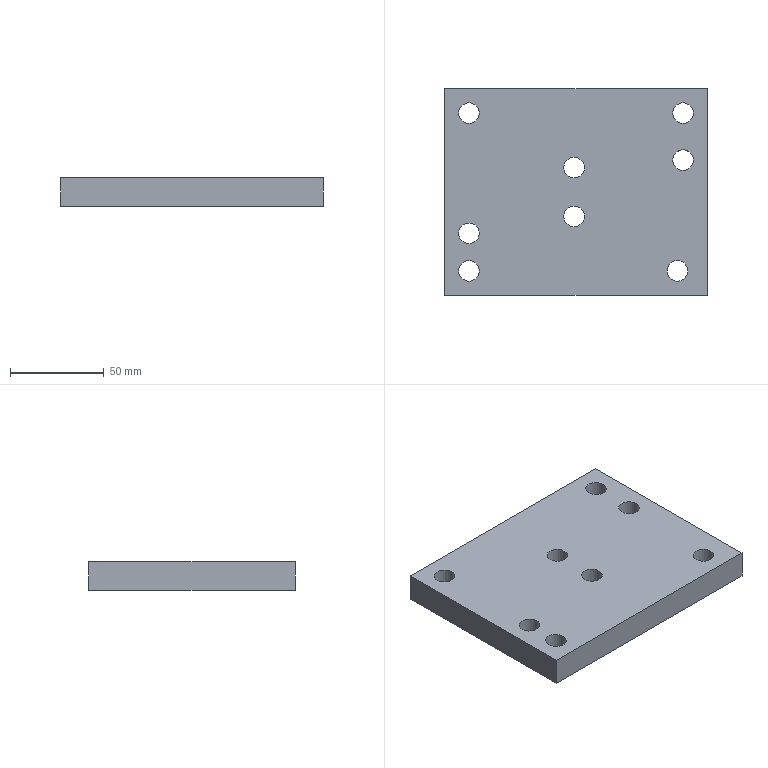Part | STEP file | 101_id682_x_t | 1 solid | 14 faces | box 140 x 110 x 15 mm | volume 219596 mm3 | cylinder 8 | plane 6 | commonest cylinder face diameters 11 x8
STEP:
#1=CARTESIAN_POINT('',(0.,0.,0.));
#2=DIRECTION('',(0.,0.,1.));
#3=DIRECTION('',(1.,0.,0.));
#4=AXIS2_PLACEMENT_3D('',#1,#2,#3);
#5=CARTESIAN_POINT('',(-791.5,35.5,105.));
#6=VERTEX_POINT('',#5);
#7=CARTESIAN_POINT('',(-791.5,35.5,90.));
#8=VERTEX_POINT('',#7);
#9=CARTESIAN_POINT('',(-791.5,35.5,95.));
#10=DIRECTION('',(0.,0.,-1.));
#11=VECTOR('',#10,1.);
#12=LINE('',#9,#11);
#13=CARTESIAN_POINT('',(-791.5,94.,95.));
#14=DIRECTION('',(-1.,0.,0.));
#15=DIRECTION('',(0.,-1.,0.));
#16=AXIS2_PLACEMENT_3D('',#13,#14,#15);
#17=PLANE('',#16);
#18=CARTESIAN_POINT('',(58.5,0.));
#19=DIRECTION('',(0.,-1.));
#20=VECTOR('',#19,1.);
#21=LINE('',#18,#20);
#22=(GEOMETRIC_REPRESENTATION_CONTEXT(2)PARAMETRIC_REPRESENTATION_CONTEXT()REPRESENTATION_CONTEXT('',''));
#23=DEFINITIONAL_REPRESENTATION('',(#21),#22);
#24=PCURVE('',#17,#23);
#25=CARTESIAN_POINT('',(-870.,35.5,95.));
#26=DIRECTION('',(0.,1.,0.));
#27=DIRECTION('',(-1.,0.,0.));
#28=AXIS2_PLACEMENT_3D('',#25,#26,#27);
#29=PLANE('',#28);
#30=CARTESIAN_POINT('',(-78.5,0.));
#31=DIRECTION('',(0.,-1.));
#32=VECTOR('',#31,1.);
#33=LINE('',#30,#32);
#34=(GEOMETRIC_REPRESENTATION_CONTEXT(2)PARAMETRIC_REPRESENTATION_CONTEXT()REPRESENTATION_CONTEXT('',''));
#35=DEFINITIONAL_REPRESENTATION('',(#33),#34);
#36=PCURVE('',#29,#35);
#37=SURFACE_CURVE('',#12,(#24,#36),.PCURVE_S1.);
#38=EDGE_CURVE('',#6,#8,#37,.T.);
#39=ORIENTED_EDGE('',*,*,#38,.T.);
#40=CARTESIAN_POINT('',(-791.5,145.5,90.));
#41=VERTEX_POINT('',#40);
#42=CARTESIAN_POINT('',(-791.5,94.,90.));
#43=DIRECTION('',(0.,-1.,0.));
#44=VECTOR('',#43,1.);
#45=LINE('',#42,#44);
#46=CARTESIAN_POINT('',(0.,-5.));
#47=DIRECTION('',(1.,0.));
#48=VECTOR('',#47,1.);
#49=LINE('',#46,#48);
#50=(GEOMETRIC_REPRESENTATION_CONTEXT(2)PARAMETRIC_REPRESENTATION_CONTEXT()REPRESENTATION_CONTEXT('',''));
#51=DEFINITIONAL_REPRESENTATION('',(#49),#50);
#52=PCURVE('',#17,#51);
#53=CARTESIAN_POINT('',(-870.,94.,90.));
#54=DIRECTION('',(0.,0.,1.));
#55=DIRECTION('',(0.,-1.,0.));
#56=AXIS2_PLACEMENT_3D('',#53,#54,#55);
#57=PLANE('',#56);
#58=CARTESIAN_POINT('',(0.,78.5));
#59=DIRECTION('',(1.,0.));
#60=VECTOR('',#59,1.);
#61=LINE('',#58,#60);
#62=(GEOMETRIC_REPRESENTATION_CONTEXT(2)PARAMETRIC_REPRESENTATION_CONTEXT()REPRESENTATION_CONTEXT('',''));
#63=DEFINITIONAL_REPRESENTATION('',(#61),#62);
#64=PCURVE('',#57,#63);
#65=SURFACE_CURVE('',#45,(#52,#64),.PCURVE_S1.);
#66=EDGE_CURVE('',#41,#8,#65,.T.);
#67=ORIENTED_EDGE('',*,*,#66,.F.);
#68=CARTESIAN_POINT('',(-791.5,145.5,105.));
#69=VERTEX_POINT('',#68);
#70=CARTESIAN_POINT('',(-791.5,145.5,95.));
#71=DIRECTION('',(0.,0.,-1.));
#72=VECTOR('',#71,1.);
#73=LINE('',#70,#72);
#74=CARTESIAN_POINT('',(-51.5,0.));
#75=DIRECTION('',(0.,-1.));
#76=VECTOR('',#75,1.);
#77=LINE('',#74,#76);
#78=(GEOMETRIC_REPRESENTATION_CONTEXT(2)PARAMETRIC_REPRESENTATION_CONTEXT()REPRESENTATION_CONTEXT('',''));
#79=DEFINITIONAL_REPRESENTATION('',(#77),#78);
#80=PCURVE('',#17,#79);
#81=CARTESIAN_POINT('',(-870.,145.5,95.));
#82=DIRECTION('',(0.,-1.,0.));
#83=DIRECTION('',(1.,0.,0.));
#84=AXIS2_PLACEMENT_3D('',#81,#82,#83);
#85=PLANE('',#84);
#86=CARTESIAN_POINT('',(78.5,0.));
#87=DIRECTION('',(0.,-1.));
#88=VECTOR('',#87,1.);
#89=LINE('',#86,#88);
#90=(GEOMETRIC_REPRESENTATION_CONTEXT(2)PARAMETRIC_REPRESENTATION_CONTEXT()REPRESENTATION_CONTEXT('',''));
#91=DEFINITIONAL_REPRESENTATION('',(#89),#90);
#92=PCURVE('',#85,#91);
#93=SURFACE_CURVE('',#73,(#80,#92),.PCURVE_S1.);
#94=EDGE_CURVE('',#69,#41,#93,.T.);
#95=ORIENTED_EDGE('',*,*,#94,.F.);
#96=CARTESIAN_POINT('',(-791.5,140.5,105.));
#97=DIRECTION('',(0.,-1.,0.));
#98=VECTOR('',#97,1.);
#99=LINE('',#96,#98);
#100=CARTESIAN_POINT('',(-46.5,10.));
#101=DIRECTION('',(1.,0.));
#102=VECTOR('',#101,1.);
#103=LINE('',#100,#102);
#104=(GEOMETRIC_REPRESENTATION_CONTEXT(2)PARAMETRIC_REPRESENTATION_CONTEXT()REPRESENTATION_CONTEXT('',''));
#105=DEFINITIONAL_REPRESENTATION('',(#103),#104);
#106=PCURVE('',#17,#105);
#107=CARTESIAN_POINT('',(-535.,140.5,105.));
#108=DIRECTION('',(0.,0.,1.));
#109=DIRECTION('',(-1.,0.,0.));
#110=AXIS2_PLACEMENT_3D('',#107,#108,#109);
#111=PLANE('',#110);
#112=CARTESIAN_POINT('',(256.5,0.));
#113=DIRECTION('',(0.,1.));
#114=VECTOR('',#113,1.);
#115=LINE('',#112,#114);
#116=(GEOMETRIC_REPRESENTATION_CONTEXT(2)PARAMETRIC_REPRESENTATION_CONTEXT()REPRESENTATION_CONTEXT('',''));
#117=DEFINITIONAL_REPRESENTATION('',(#115),#116);
#118=PCURVE('',#111,#117);
#119=SURFACE_CURVE('',#99,(#106,#118),.PCURVE_S1.);
#120=EDGE_CURVE('',#69,#6,#119,.T.);
#121=ORIENTED_EDGE('',*,*,#120,.T.);
#122=EDGE_LOOP('',(#39,#67,#95,#121));
#123=FACE_BOUND('',#122,.T.);
#124=ADVANCED_FACE('',(#123),#17,.F.);
#125=ORIENTED_EDGE('',*,*,#94,.T.);
#126=CARTESIAN_POINT('',(-931.5,145.5,90.));
#127=VERTEX_POINT('',#126);
#128=CARTESIAN_POINT('',(-870.,145.5,90.));
#129=DIRECTION('',(1.,0.,0.));
#130=VECTOR('',#129,1.);
#131=LINE('',#128,#130);
#132=CARTESIAN_POINT('',(0.,-5.));
#133=DIRECTION('',(1.,0.));
#134=VECTOR('',#133,1.);
#135=LINE('',#132,#134);
#136=(GEOMETRIC_REPRESENTATION_CONTEXT(2)PARAMETRIC_REPRESENTATION_CONTEXT()REPRESENTATION_CONTEXT('',''));
#137=DEFINITIONAL_REPRESENTATION('',(#135),#136);
#138=PCURVE('',#85,#137);
#139=CARTESIAN_POINT('',(-51.5,0.));
#140=DIRECTION('',(0.,1.));
#141=VECTOR('',#140,1.);
#142=LINE('',#139,#141);
#143=(GEOMETRIC_REPRESENTATION_CONTEXT(2)PARAMETRIC_REPRESENTATION_CONTEXT()REPRESENTATION_CONTEXT('',''));
#144=DEFINITIONAL_REPRESENTATION('',(#142),#143);
#145=PCURVE('',#57,#144);
#146=SURFACE_CURVE('',#131,(#138,#145),.PCURVE_S1.);
#147=EDGE_CURVE('',#127,#41,#146,.T.);
#148=ORIENTED_EDGE('',*,*,#147,.F.);
#149=CARTESIAN_POINT('',(-931.5,145.5,105.));
#150=VERTEX_POINT('',#149);
#151=CARTESIAN_POINT('',(-931.5,145.5,95.));
#152=DIRECTION('',(0.,0.,-1.));
#153=VECTOR('',#152,1.);
#154=LINE('',#151,#153);
#155=CARTESIAN_POINT('',(-61.5,0.));
#156=DIRECTION('',(0.,-1.));
#157=VECTOR('',#156,1.);
#158=LINE('',#155,#157);
#159=(GEOMETRIC_REPRESENTATION_CONTEXT(2)PARAMETRIC_REPRESENTATION_CONTEXT()REPRESENTATION_CONTEXT('',''));
#160=DEFINITIONAL_REPRESENTATION('',(#158),#159);
#161=PCURVE('',#85,#160);
#162=CARTESIAN_POINT('',(-931.5,94.,95.));
#163=DIRECTION('',(1.,0.,0.));
#164=DIRECTION('',(0.,1.,0.));
#165=AXIS2_PLACEMENT_3D('',#162,#163,#164);
#166=PLANE('',#165);
#167=CARTESIAN_POINT('',(51.5,0.));
#168=DIRECTION('',(0.,-1.));
#169=VECTOR('',#168,1.);
#170=LINE('',#167,#169);
#171=(GEOMETRIC_REPRESENTATION_CONTEXT(2)PARAMETRIC_REPRESENTATION_CONTEXT()REPRESENTATION_CONTEXT('',''));
#172=DEFINITIONAL_REPRESENTATION('',(#170),#171);
#173=PCURVE('',#166,#172);
#174=SURFACE_CURVE('',#154,(#161,#173),.PCURVE_S1.);
#175=EDGE_CURVE('',#150,#127,#174,.T.);
#176=ORIENTED_EDGE('',*,*,#175,.F.);
#177=CARTESIAN_POINT('',(-535.,145.5,105.));
#178=DIRECTION('',(1.,0.,0.));
#179=VECTOR('',#178,1.);
#180=LINE('',#177,#179);
#181=CARTESIAN_POINT('',(335.,10.));
#182=DIRECTION('',(1.,0.));
#183=VECTOR('',#182,1.);
#184=LINE('',#181,#183);
#185=(GEOMETRIC_REPRESENTATION_CONTEXT(2)PARAMETRIC_REPRESENTATION_CONTEXT()REPRESENTATION_CONTEXT('',''));
#186=DEFINITIONAL_REPRESENTATION('',(#184),#185);
#187=PCURVE('',#85,#186);
#188=CARTESIAN_POINT('',(0.,-5.));
#189=DIRECTION('',(-1.,0.));
#190=VECTOR('',#189,1.);
#191=LINE('',#188,#190);
#192=(GEOMETRIC_REPRESENTATION_CONTEXT(2)PARAMETRIC_REPRESENTATION_CONTEXT()REPRESENTATION_CONTEXT('',''));
#193=DEFINITIONAL_REPRESENTATION('',(#191),#192);
#194=PCURVE('',#111,#193);
#195=SURFACE_CURVE('',#180,(#187,#194),.PCURVE_S1.);
#196=EDGE_CURVE('',#150,#69,#195,.T.);
#197=ORIENTED_EDGE('',*,*,#196,.T.);
#198=EDGE_LOOP('',(#125,#148,#176,#197));
#199=FACE_BOUND('',#198,.T.);
#200=ADVANCED_FACE('',(#199),#85,.F.);
#201=ORIENTED_EDGE('',*,*,#175,.T.);
#202=CARTESIAN_POINT('',(-931.5,35.5,90.));
#203=VERTEX_POINT('',#202);
#204=CARTESIAN_POINT('',(-931.5,94.,90.));
#205=DIRECTION('',(0.,1.,0.));
#206=VECTOR('',#205,1.);
#207=LINE('',#204,#206);
#208=CARTESIAN_POINT('',(0.,-5.));
#209=DIRECTION('',(1.,0.));
#210=VECTOR('',#209,1.);
#211=LINE('',#208,#210);
#212=(GEOMETRIC_REPRESENTATION_CONTEXT(2)PARAMETRIC_REPRESENTATION_CONTEXT()REPRESENTATION_CONTEXT('',''));
#213=DEFINITIONAL_REPRESENTATION('',(#211),#212);
#214=PCURVE('',#166,#213);
#215=CARTESIAN_POINT('',(0.,-61.5));
#216=DIRECTION('',(-1.,0.));
#217=VECTOR('',#216,1.);
#218=LINE('',#215,#217);
#219=(GEOMETRIC_REPRESENTATION_CONTEXT(2)PARAMETRIC_REPRESENTATION_CONTEXT()REPRESENTATION_CONTEXT('',''));
#220=DEFINITIONAL_REPRESENTATION('',(#218),#219);
#221=PCURVE('',#57,#220);
#222=SURFACE_CURVE('',#207,(#214,#221),.PCURVE_S1.);
#223=EDGE_CURVE('',#203,#127,#222,.T.);
#224=ORIENTED_EDGE('',*,*,#223,.F.);
#225=CARTESIAN_POINT('',(-931.5,35.5,105.));
#226=VERTEX_POINT('',#225);
#227=CARTESIAN_POINT('',(-931.5,35.5,95.));
#228=DIRECTION('',(0.,0.,-1.));
#229=VECTOR('',#228,1.);
#230=LINE('',#227,#229);
#231=CARTESIAN_POINT('',(-58.5,0.));
#232=DIRECTION('',(0.,-1.));
#233=VECTOR('',#232,1.);
#234=LINE('',#231,#233);
#235=(GEOMETRIC_REPRESENTATION_CONTEXT(2)PARAMETRIC_REPRESENTATION_CONTEXT()REPRESENTATION_CONTEXT('',''));
#236=DEFINITIONAL_REPRESENTATION('',(#234),#235);
#237=PCURVE('',#166,#236);
#238=CARTESIAN_POINT('',(61.5,0.));
#239=DIRECTION('',(0.,-1.));
#240=VECTOR('',#239,1.);
#241=LINE('',#238,#240);
#242=(GEOMETRIC_REPRESENTATION_CONTEXT(2)PARAMETRIC_REPRESENTATION_CONTEXT()REPRESENTATION_CONTEXT('',''));
#243=DEFINITIONAL_REPRESENTATION('',(#241),#242);
#244=PCURVE('',#29,#243);
#245=SURFACE_CURVE('',#230,(#237,#244),.PCURVE_S1.);
#246=EDGE_CURVE('',#226,#203,#245,.T.);
#247=ORIENTED_EDGE('',*,*,#246,.F.);
#248=CARTESIAN_POINT('',(-931.5,140.5,105.));
#249=DIRECTION('',(0.,1.,0.));
#250=VECTOR('',#249,1.);
#251=LINE('',#248,#250);
#252=CARTESIAN_POINT('',(46.5,10.));
#253=DIRECTION('',(1.,0.));
#254=VECTOR('',#253,1.);
#255=LINE('',#252,#254);
#256=(GEOMETRIC_REPRESENTATION_CONTEXT(2)PARAMETRIC_REPRESENTATION_CONTEXT()REPRESENTATION_CONTEXT('',''));
#257=DEFINITIONAL_REPRESENTATION('',(#255),#256);
#258=PCURVE('',#166,#257);
#259=CARTESIAN_POINT('',(396.5,0.));
#260=DIRECTION('',(0.,-1.));
#261=VECTOR('',#260,1.);
#262=LINE('',#259,#261);
#263=(GEOMETRIC_REPRESENTATION_CONTEXT(2)PARAMETRIC_REPRESENTATION_CONTEXT()REPRESENTATION_CONTEXT('',''));
#264=DEFINITIONAL_REPRESENTATION('',(#262),#263);
#265=PCURVE('',#111,#264);
#266=SURFACE_CURVE('',#251,(#258,#265),.PCURVE_S1.);
#267=EDGE_CURVE('',#226,#150,#266,.T.);
#268=ORIENTED_EDGE('',*,*,#267,.T.);
#269=EDGE_LOOP('',(#201,#224,#247,#268));
#270=FACE_BOUND('',#269,.T.);
#271=ADVANCED_FACE('',(#270),#166,.F.);
#272=CARTESIAN_POINT('',(-799.,132.5,90.));
#273=VERTEX_POINT('',#272);
#274=CARTESIAN_POINT('',(-804.5,132.5,90.));
#275=DIRECTION('',(0.,0.,-1.));
#276=DIRECTION('',(1.,0.,0.));
#277=AXIS2_PLACEMENT_3D('',#274,#275,#276);
#278=CIRCLE('',#277,5.5);
#279=CARTESIAN_POINT('',(-804.5,132.5,95.));
#280=DIRECTION('',(0.,0.,1.));
#281=DIRECTION('',(1.,0.,0.));
#282=AXIS2_PLACEMENT_3D('',#279,#280,#281);
#283=CYLINDRICAL_SURFACE('',#282,5.5);
#284=CARTESIAN_POINT('',(6.283,-5.));
#285=DIRECTION('',(-1.,0.));
#286=VECTOR('',#285,1.);
#287=LINE('',#284,#286);
#288=(GEOMETRIC_REPRESENTATION_CONTEXT(2)PARAMETRIC_REPRESENTATION_CONTEXT()REPRESENTATION_CONTEXT('',''));
#289=DEFINITIONAL_REPRESENTATION('',(#287),#288);
#290=PCURVE('',#283,#289);
#291=CARTESIAN_POINT('',(-38.5,71.));
#292=CARTESIAN_POINT('',(-28.974,71.));
#293=CARTESIAN_POINT('',(-33.737,62.75));
#294=CARTESIAN_POINT('',(-38.5,54.5));
#295=CARTESIAN_POINT('',(-43.263,62.75));
#296=CARTESIAN_POINT('',(-48.026,71.));
#297=CARTESIAN_POINT('',(-38.5,71.));
#298=(BOUNDED_CURVE()B_SPLINE_CURVE(2,(#291,#292,#293,#294,#295,#296,#297),.UNSPECIFIED.,.T.,.F.)B_SPLINE_CURVE_WITH_KNOTS((1,2,2,2,2,1),(-2.094,0.,2.094,4.189,6.283,8.378),.UNSPECIFIED.)CURVE()GEOMETRIC_REPRESENTATION_ITEM()RATIONAL_B_SPLINE_CURVE((1.,0.5,1.,0.5,1.,0.5,1.))REPRESENTATION_ITEM(''));
#299=(GEOMETRIC_REPRESENTATION_CONTEXT(2)PARAMETRIC_REPRESENTATION_CONTEXT()REPRESENTATION_CONTEXT('',''));
#300=DEFINITIONAL_REPRESENTATION('',(#298),#299);
#301=PCURVE('',#57,#300);
#302=SURFACE_CURVE('',#278,(#290,#301),.PCURVE_S1.);
#303=EDGE_CURVE('',#273,#273,#302,.T.);
#304=ORIENTED_EDGE('',*,*,#303,.F.);
#305=CARTESIAN_POINT('',(-799.,132.5,105.));
#306=VERTEX_POINT('',#305);
#307=CARTESIAN_POINT('',(-799.,132.5,90.));
#308=CARTESIAN_POINT('',(-799.,132.5,105.));
#309=B_SPLINE_CURVE_WITH_KNOTS('',1,(#307,#308),.UNSPECIFIED.,.F.,.F.,(2,2),(-5.,10.),.PIECEWISE_BEZIER_KNOTS.);
#310=CARTESIAN_POINT('',(6.283,0.));
#311=DIRECTION('',(0.,1.));
#312=VECTOR('',#311,1.);
#313=LINE('',#310,#312);
#314=(GEOMETRIC_REPRESENTATION_CONTEXT(2)PARAMETRIC_REPRESENTATION_CONTEXT()REPRESENTATION_CONTEXT('',''));
#315=DEFINITIONAL_REPRESENTATION('',(#313),#314);
#316=PCURVE('',#283,#315);
#317=CARTESIAN_POINT('',(0.,0.));
#318=DIRECTION('',(0.,1.));
#319=VECTOR('',#318,1.);
#320=LINE('',#317,#319);
#321=(GEOMETRIC_REPRESENTATION_CONTEXT(2)PARAMETRIC_REPRESENTATION_CONTEXT()REPRESENTATION_CONTEXT('',''));
#322=DEFINITIONAL_REPRESENTATION('',(#320),#321);
#323=PCURVE('',#283,#322);
#324=SEAM_CURVE('',#309,(#316,#323),.PCURVE_S1.);
#325=EDGE_CURVE('',#273,#306,#324,.T.);
#326=ORIENTED_EDGE('',*,*,#325,.T.);
#327=CARTESIAN_POINT('',(-804.5,132.5,105.));
#328=DIRECTION('',(0.,0.,-1.));
#329=DIRECTION('',(1.,0.,0.));
#330=AXIS2_PLACEMENT_3D('',#327,#328,#329);
#331=CIRCLE('',#330,5.5);
#332=CARTESIAN_POINT('',(6.283,10.));
#333=DIRECTION('',(-1.,0.));
#334=VECTOR('',#333,1.);
#335=LINE('',#332,#334);
#336=(GEOMETRIC_REPRESENTATION_CONTEXT(2)PARAMETRIC_REPRESENTATION_CONTEXT()REPRESENTATION_CONTEXT('',''));
#337=DEFINITIONAL_REPRESENTATION('',(#335),#336);
#338=PCURVE('',#283,#337);
#339=CARTESIAN_POINT('',(264.,8.));
#340=CARTESIAN_POINT('',(264.,17.526));
#341=CARTESIAN_POINT('',(272.25,12.763));
#342=CARTESIAN_POINT('',(280.5,8.));
#343=CARTESIAN_POINT('',(272.25,3.237));
#344=CARTESIAN_POINT('',(264.,-1.526));
#345=CARTESIAN_POINT('',(264.,8.));
#346=(BOUNDED_CURVE()B_SPLINE_CURVE(2,(#339,#340,#341,#342,#343,#344,#345),.UNSPECIFIED.,.T.,.F.)B_SPLINE_CURVE_WITH_KNOTS((1,2,2,2,2,1),(-2.094,0.,2.094,4.189,6.283,8.378),.UNSPECIFIED.)CURVE()GEOMETRIC_REPRESENTATION_ITEM()RATIONAL_B_SPLINE_CURVE((1.,0.5,1.,0.5,1.,0.5,1.))REPRESENTATION_ITEM(''));
#347=(GEOMETRIC_REPRESENTATION_CONTEXT(2)PARAMETRIC_REPRESENTATION_CONTEXT()REPRESENTATION_CONTEXT('',''));
#348=DEFINITIONAL_REPRESENTATION('',(#346),#347);
#349=PCURVE('',#111,#348);
#350=SURFACE_CURVE('',#331,(#338,#349),.PCURVE_S1.);
#351=EDGE_CURVE('',#306,#306,#350,.T.);
#352=ORIENTED_EDGE('',*,*,#351,.T.);
#353=ORIENTED_EDGE('',*,*,#325,.F.);
#354=EDGE_LOOP('',(#304,#326,#352,#353));
#355=FACE_BOUND('',#354,.F.);
#356=ADVANCED_FACE('',(#355),#283,.F.);
#357=CARTESIAN_POINT('',(-535.,35.5,105.));
#358=DIRECTION('',(-1.,0.,0.));
#359=VECTOR('',#358,1.);
#360=LINE('',#357,#359);
#361=CARTESIAN_POINT('',(-335.,10.));
#362=DIRECTION('',(1.,0.));
#363=VECTOR('',#362,1.);
#364=LINE('',#361,#363);
#365=(GEOMETRIC_REPRESENTATION_CONTEXT(2)PARAMETRIC_REPRESENTATION_CONTEXT()REPRESENTATION_CONTEXT('',''));
#366=DEFINITIONAL_REPRESENTATION('',(#364),#365);
#367=PCURVE('',#29,#366);
#368=CARTESIAN_POINT('',(0.,105.));
#369=DIRECTION('',(1.,0.));
#370=VECTOR('',#369,1.);
#371=LINE('',#368,#370);
#372=(GEOMETRIC_REPRESENTATION_CONTEXT(2)PARAMETRIC_REPRESENTATION_CONTEXT()REPRESENTATION_CONTEXT('',''));
#373=DEFINITIONAL_REPRESENTATION('',(#371),#372);
#374=PCURVE('',#111,#373);
#375=SURFACE_CURVE('',#360,(#367,#374),.PCURVE_S1.);
#376=EDGE_CURVE('',#6,#226,#375,.T.);
#377=ORIENTED_EDGE('',*,*,#376,.T.);
#378=ORIENTED_EDGE('',*,*,#246,.T.);
#379=CARTESIAN_POINT('',(-870.,35.5,90.));
#380=DIRECTION('',(-1.,0.,0.));
#381=VECTOR('',#380,1.);
#382=LINE('',#379,#381);
#383=CARTESIAN_POINT('',(0.,-5.));
#384=DIRECTION('',(1.,0.));
#385=VECTOR('',#384,1.);
#386=LINE('',#383,#385);
#387=(GEOMETRIC_REPRESENTATION_CONTEXT(2)PARAMETRIC_REPRESENTATION_CONTEXT()REPRESENTATION_CONTEXT('',''));
#388=DEFINITIONAL_REPRESENTATION('',(#386),#387);
#389=PCURVE('',#29,#388);
#390=CARTESIAN_POINT('',(58.5,0.));
#391=DIRECTION('',(0.,-1.));
#392=VECTOR('',#391,1.);
#393=LINE('',#390,#392);
#394=(GEOMETRIC_REPRESENTATION_CONTEXT(2)PARAMETRIC_REPRESENTATION_CONTEXT()REPRESENTATION_CONTEXT('',''));
#395=DEFINITIONAL_REPRESENTATION('',(#393),#394);
#396=PCURVE('',#57,#395);
#397=SURFACE_CURVE('',#382,(#389,#396),.PCURVE_S1.);
#398=EDGE_CURVE('',#8,#203,#397,.T.);
#399=ORIENTED_EDGE('',*,*,#398,.F.);
#400=ORIENTED_EDGE('',*,*,#38,.F.);
#401=EDGE_LOOP('',(#377,#378,#399,#400));
#402=FACE_BOUND('',#401,.T.);
#403=ADVANCED_FACE('',(#402),#29,.F.);
#404=CARTESIAN_POINT('',(-913.,132.5,90.));
#405=VERTEX_POINT('',#404);
#406=CARTESIAN_POINT('',(-918.5,132.5,90.));
#407=DIRECTION('',(0.,0.,-1.));
#408=DIRECTION('',(1.,0.,0.));
#409=AXIS2_PLACEMENT_3D('',#406,#407,#408);
#410=CIRCLE('',#409,5.5);
#411=CARTESIAN_POINT('',(-918.5,132.5,95.));
#412=DIRECTION('',(0.,0.,1.));
#413=DIRECTION('',(1.,0.,0.));
#414=AXIS2_PLACEMENT_3D('',#411,#412,#413);
#415=CYLINDRICAL_SURFACE('',#414,5.5);
#416=CARTESIAN_POINT('',(6.283,-5.));
#417=DIRECTION('',(-1.,0.));
#418=VECTOR('',#417,1.);
#419=LINE('',#416,#418);
#420=(GEOMETRIC_REPRESENTATION_CONTEXT(2)PARAMETRIC_REPRESENTATION_CONTEXT()REPRESENTATION_CONTEXT('',''));
#421=DEFINITIONAL_REPRESENTATION('',(#419),#420);
#422=PCURVE('',#415,#421);
#423=CARTESIAN_POINT('',(-38.5,-43.));
#424=CARTESIAN_POINT('',(-28.974,-43.));
#425=CARTESIAN_POINT('',(-33.737,-51.25));
#426=CARTESIAN_POINT('',(-38.5,-59.5));
#427=CARTESIAN_POINT('',(-43.263,-51.25));
#428=CARTESIAN_POINT('',(-48.026,-43.));
#429=CARTESIAN_POINT('',(-38.5,-43.));
#430=(BOUNDED_CURVE()B_SPLINE_CURVE(2,(#423,#424,#425,#426,#427,#428,#429),.UNSPECIFIED.,.T.,.F.)B_SPLINE_CURVE_WITH_KNOTS((1,2,2,2,2,1),(-2.094,0.,2.094,4.189,6.283,8.378),.UNSPECIFIED.)CURVE()GEOMETRIC_REPRESENTATION_ITEM()RATIONAL_B_SPLINE_CURVE((1.,0.5,1.,0.5,1.,0.5,1.))REPRESENTATION_ITEM(''));
#431=(GEOMETRIC_REPRESENTATION_CONTEXT(2)PARAMETRIC_REPRESENTATION_CONTEXT()REPRESENTATION_CONTEXT('',''));
#432=DEFINITIONAL_REPRESENTATION('',(#430),#431);
#433=PCURVE('',#57,#432);
#434=SURFACE_CURVE('',#410,(#422,#433),.PCURVE_S1.);
#435=EDGE_CURVE('',#405,#405,#434,.T.);
#436=ORIENTED_EDGE('',*,*,#435,.F.);
#437=CARTESIAN_POINT('',(-913.,132.5,105.));
#438=VERTEX_POINT('',#437);
#439=CARTESIAN_POINT('',(-913.,132.5,90.));
#440=CARTESIAN_POINT('',(-913.,132.5,105.));
#441=B_SPLINE_CURVE_WITH_KNOTS('',1,(#439,#440),.UNSPECIFIED.,.F.,.F.,(2,2),(-5.,10.),.PIECEWISE_BEZIER_KNOTS.);
#442=CARTESIAN_POINT('',(6.283,0.));
#443=DIRECTION('',(0.,1.));
#444=VECTOR('',#443,1.);
#445=LINE('',#442,#444);
#446=(GEOMETRIC_REPRESENTATION_CONTEXT(2)PARAMETRIC_REPRESENTATION_CONTEXT()REPRESENTATION_CONTEXT('',''));
#447=DEFINITIONAL_REPRESENTATION('',(#445),#446);
#448=PCURVE('',#415,#447);
#449=CARTESIAN_POINT('',(0.,0.));
#450=DIRECTION('',(0.,1.));
#451=VECTOR('',#450,1.);
#452=LINE('',#449,#451);
#453=(GEOMETRIC_REPRESENTATION_CONTEXT(2)PARAMETRIC_REPRESENTATION_CONTEXT()REPRESENTATION_CONTEXT('',''));
#454=DEFINITIONAL_REPRESENTATION('',(#452),#453);
#455=PCURVE('',#415,#454);
#456=SEAM_CURVE('',#441,(#448,#455),.PCURVE_S1.);
#457=EDGE_CURVE('',#405,#438,#456,.T.);
#458=ORIENTED_EDGE('',*,*,#457,.T.);
#459=CARTESIAN_POINT('',(-918.5,132.5,105.));
#460=DIRECTION('',(0.,0.,-1.));
#461=DIRECTION('',(1.,0.,0.));
#462=AXIS2_PLACEMENT_3D('',#459,#460,#461);
#463=CIRCLE('',#462,5.5);
#464=CARTESIAN_POINT('',(6.283,10.));
#465=DIRECTION('',(-1.,0.));
#466=VECTOR('',#465,1.);
#467=LINE('',#464,#466);
#468=(GEOMETRIC_REPRESENTATION_CONTEXT(2)PARAMETRIC_REPRESENTATION_CONTEXT()REPRESENTATION_CONTEXT('',''));
#469=DEFINITIONAL_REPRESENTATION('',(#467),#468);
#470=PCURVE('',#415,#469);
#471=CARTESIAN_POINT('',(378.,8.));
#472=CARTESIAN_POINT('',(378.,17.526));
#473=CARTESIAN_POINT('',(386.25,12.763));
#474=CARTESIAN_POINT('',(394.5,8.));
#475=CARTESIAN_POINT('',(386.25,3.237));
#476=CARTESIAN_POINT('',(378.,-1.526));
#477=CARTESIAN_POINT('',(378.,8.));
#478=(BOUNDED_CURVE()B_SPLINE_CURVE(2,(#471,#472,#473,#474,#475,#476,#477),.UNSPECIFIED.,.T.,.F.)B_SPLINE_CURVE_WITH_KNOTS((1,2,2,2,2,1),(-2.094,0.,2.094,4.189,6.283,8.378),.UNSPECIFIED.)CURVE()GEOMETRIC_REPRESENTATION_ITEM()RATIONAL_B_SPLINE_CURVE((1.,0.5,1.,0.5,1.,0.5,1.))REPRESENTATION_ITEM(''));
#479=(GEOMETRIC_REPRESENTATION_CONTEXT(2)PARAMETRIC_REPRESENTATION_CONTEXT()REPRESENTATION_CONTEXT('',''));
#480=DEFINITIONAL_REPRESENTATION('',(#478),#479);
#481=PCURVE('',#111,#480);
#482=SURFACE_CURVE('',#463,(#470,#481),.PCURVE_S1.);
#483=EDGE_CURVE('',#438,#438,#482,.T.);
#484=ORIENTED_EDGE('',*,*,#483,.T.);
#485=ORIENTED_EDGE('',*,*,#457,.F.);
#486=EDGE_LOOP('',(#436,#458,#484,#485));
#487=FACE_BOUND('',#486,.F.);
#488=ADVANCED_FACE('',(#487),#415,.F.);
#489=CARTESIAN_POINT('',(-913.,48.5,90.));
#490=VERTEX_POINT('',#489);
#491=CARTESIAN_POINT('',(-918.5,48.5,90.));
#492=DIRECTION('',(0.,0.,-1.));
#493=DIRECTION('',(1.,0.,0.));
#494=AXIS2_PLACEMENT_3D('',#491,#492,#493);
#495=CIRCLE('',#494,5.5);
#496=CARTESIAN_POINT('',(-918.5,48.5,95.));
#497=DIRECTION('',(0.,0.,1.));
#498=DIRECTION('',(1.,0.,0.));
#499=AXIS2_PLACEMENT_3D('',#496,#497,#498);
#500=CYLINDRICAL_SURFACE('',#499,5.5);
#501=CARTESIAN_POINT('',(6.283,-5.));
#502=DIRECTION('',(-1.,0.));
#503=VECTOR('',#502,1.);
#504=LINE('',#501,#503);
#505=(GEOMETRIC_REPRESENTATION_CONTEXT(2)PARAMETRIC_REPRESENTATION_CONTEXT()REPRESENTATION_CONTEXT('',''));
#506=DEFINITIONAL_REPRESENTATION('',(#504),#505);
#507=PCURVE('',#500,#506);
#508=CARTESIAN_POINT('',(45.5,-43.));
#509=CARTESIAN_POINT('',(55.026,-43.));
#510=CARTESIAN_POINT('',(50.263,-51.25));
#511=CARTESIAN_POINT('',(45.5,-59.5));
#512=CARTESIAN_POINT('',(40.737,-51.25));
#513=CARTESIAN_POINT('',(35.974,-43.));
#514=CARTESIAN_POINT('',(45.5,-43.));
#515=(BOUNDED_CURVE()B_SPLINE_CURVE(2,(#508,#509,#510,#511,#512,#513,#514),.UNSPECIFIED.,.T.,.F.)B_SPLINE_CURVE_WITH_KNOTS((1,2,2,2,2,1),(-2.094,0.,2.094,4.189,6.283,8.378),.UNSPECIFIED.)CURVE()GEOMETRIC_REPRESENTATION_ITEM()RATIONAL_B_SPLINE_CURVE((1.,0.5,1.,0.5,1.,0.5,1.))REPRESENTATION_ITEM(''));
#516=(GEOMETRIC_REPRESENTATION_CONTEXT(2)PARAMETRIC_REPRESENTATION_CONTEXT()REPRESENTATION_CONTEXT('',''));
#517=DEFINITIONAL_REPRESENTATION('',(#515),#516);
#518=PCURVE('',#57,#517);
#519=SURFACE_CURVE('',#495,(#507,#518),.PCURVE_S1.);
#520=EDGE_CURVE('',#490,#490,#519,.T.);
#521=ORIENTED_EDGE('',*,*,#520,.F.);
#522=CARTESIAN_POINT('',(-913.,48.5,105.));
#523=VERTEX_POINT('',#522);
#524=CARTESIAN_POINT('',(-913.,48.5,90.));
#525=CARTESIAN_POINT('',(-913.,48.5,105.));
#526=B_SPLINE_CURVE_WITH_KNOTS('',1,(#524,#525),.UNSPECIFIED.,.F.,.F.,(2,2),(-5.,10.),.PIECEWISE_BEZIER_KNOTS.);
#527=CARTESIAN_POINT('',(6.283,0.));
#528=DIRECTION('',(0.,1.));
#529=VECTOR('',#528,1.);
#530=LINE('',#527,#529);
#531=(GEOMETRIC_REPRESENTATION_CONTEXT(2)PARAMETRIC_REPRESENTATION_CONTEXT()REPRESENTATION_CONTEXT('',''));
#532=DEFINITIONAL_REPRESENTATION('',(#530),#531);
#533=PCURVE('',#500,#532);
#534=CARTESIAN_POINT('',(0.,0.));
#535=DIRECTION('',(0.,1.));
#536=VECTOR('',#535,1.);
#537=LINE('',#534,#536);
#538=(GEOMETRIC_REPRESENTATION_CONTEXT(2)PARAMETRIC_REPRESENTATION_CONTEXT()REPRESENTATION_CONTEXT('',''));
#539=DEFINITIONAL_REPRESENTATION('',(#537),#538);
#540=PCURVE('',#500,#539);
#541=SEAM_CURVE('',#526,(#533,#540),.PCURVE_S1.);
#542=EDGE_CURVE('',#490,#523,#541,.T.);
#543=ORIENTED_EDGE('',*,*,#542,.T.);
#544=CARTESIAN_POINT('',(-918.5,48.5,105.));
#545=DIRECTION('',(0.,0.,-1.));
#546=DIRECTION('',(1.,0.,0.));
#547=AXIS2_PLACEMENT_3D('',#544,#545,#546);
#548=CIRCLE('',#547,5.5);
#549=CARTESIAN_POINT('',(6.283,10.));
#550=DIRECTION('',(-1.,0.));
#551=VECTOR('',#550,1.);
#552=LINE('',#549,#551);
#553=(GEOMETRIC_REPRESENTATION_CONTEXT(2)PARAMETRIC_REPRESENTATION_CONTEXT()REPRESENTATION_CONTEXT('',''));
#554=DEFINITIONAL_REPRESENTATION('',(#552),#553);
#555=PCURVE('',#500,#554);
#556=CARTESIAN_POINT('',(378.,92.));
#557=CARTESIAN_POINT('',(378.,101.526));
#558=CARTESIAN_POINT('',(386.25,96.763));
#559=CARTESIAN_POINT('',(394.5,92.));
#560=CARTESIAN_POINT('',(386.25,87.237));
#561=CARTESIAN_POINT('',(378.,82.474));
#562=CARTESIAN_POINT('',(378.,92.));
#563=(BOUNDED_CURVE()B_SPLINE_CURVE(2,(#556,#557,#558,#559,#560,#561,#562),.UNSPECIFIED.,.T.,.F.)B_SPLINE_CURVE_WITH_KNOTS((1,2,2,2,2,1),(-2.094,0.,2.094,4.189,6.283,8.378),.UNSPECIFIED.)CURVE()GEOMETRIC_REPRESENTATION_ITEM()RATIONAL_B_SPLINE_CURVE((1.,0.5,1.,0.5,1.,0.5,1.))REPRESENTATION_ITEM(''));
#564=(GEOMETRIC_REPRESENTATION_CONTEXT(2)PARAMETRIC_REPRESENTATION_CONTEXT()REPRESENTATION_CONTEXT('',''));
#565=DEFINITIONAL_REPRESENTATION('',(#563),#564);
#566=PCURVE('',#111,#565);
#567=SURFACE_CURVE('',#548,(#555,#566),.PCURVE_S1.);
#568=EDGE_CURVE('',#523,#523,#567,.T.);
#569=ORIENTED_EDGE('',*,*,#568,.T.);
#570=ORIENTED_EDGE('',*,*,#542,.F.);
#571=EDGE_LOOP('',(#521,#543,#569,#570));
#572=FACE_BOUND('',#571,.F.);
#573=ADVANCED_FACE('',(#572),#500,.F.);
#574=CARTESIAN_POINT('',(-913.,68.5,90.));
#575=VERTEX_POINT('',#574);
#576=CARTESIAN_POINT('',(-918.5,68.5,90.));
#577=DIRECTION('',(0.,0.,-1.));
#578=DIRECTION('',(1.,0.,0.));
#579=AXIS2_PLACEMENT_3D('',#576,#577,#578);
#580=CIRCLE('',#579,5.5);
#581=CARTESIAN_POINT('',(-918.5,68.5,95.));
#582=DIRECTION('',(0.,0.,1.));
#583=DIRECTION('',(1.,0.,0.));
#584=AXIS2_PLACEMENT_3D('',#581,#582,#583);
#585=CYLINDRICAL_SURFACE('',#584,5.5);
#586=CARTESIAN_POINT('',(6.283,-5.));
#587=DIRECTION('',(-1.,0.));
#588=VECTOR('',#587,1.);
#589=LINE('',#586,#588);
#590=(GEOMETRIC_REPRESENTATION_CONTEXT(2)PARAMETRIC_REPRESENTATION_CONTEXT()REPRESENTATION_CONTEXT('',''));
#591=DEFINITIONAL_REPRESENTATION('',(#589),#590);
#592=PCURVE('',#585,#591);
#593=CARTESIAN_POINT('',(25.5,-43.));
#594=CARTESIAN_POINT('',(35.026,-43.));
#595=CARTESIAN_POINT('',(30.263,-51.25));
#596=CARTESIAN_POINT('',(25.5,-59.5));
#597=CARTESIAN_POINT('',(20.737,-51.25));
#598=CARTESIAN_POINT('',(15.974,-43.));
#599=CARTESIAN_POINT('',(25.5,-43.));
#600=(BOUNDED_CURVE()B_SPLINE_CURVE(2,(#593,#594,#595,#596,#597,#598,#599),.UNSPECIFIED.,.T.,.F.)B_SPLINE_CURVE_WITH_KNOTS((1,2,2,2,2,1),(-2.094,0.,2.094,4.189,6.283,8.378),.UNSPECIFIED.)CURVE()GEOMETRIC_REPRESENTATION_ITEM()RATIONAL_B_SPLINE_CURVE((1.,0.5,1.,0.5,1.,0.5,1.))REPRESENTATION_ITEM(''));
#601=(GEOMETRIC_REPRESENTATION_CONTEXT(2)PARAMETRIC_REPRESENTATION_CONTEXT()REPRESENTATION_CONTEXT('',''));
#602=DEFINITIONAL_REPRESENTATION('',(#600),#601);
#603=PCURVE('',#57,#602);
#604=SURFACE_CURVE('',#580,(#592,#603),.PCURVE_S1.);
#605=EDGE_CURVE('',#575,#575,#604,.T.);
#606=ORIENTED_EDGE('',*,*,#605,.F.);
#607=CARTESIAN_POINT('',(-913.,68.5,105.));
#608=VERTEX_POINT('',#607);
#609=CARTESIAN_POINT('',(-913.,68.5,90.));
#610=CARTESIAN_POINT('',(-913.,68.5,105.));
#611=B_SPLINE_CURVE_WITH_KNOTS('',1,(#609,#610),.UNSPECIFIED.,.F.,.F.,(2,2),(-5.,10.),.PIECEWISE_BEZIER_KNOTS.);
#612=CARTESIAN_POINT('',(6.283,0.));
#613=DIRECTION('',(0.,1.));
#614=VECTOR('',#613,1.);
#615=LINE('',#612,#614);
#616=(GEOMETRIC_REPRESENTATION_CONTEXT(2)PARAMETRIC_REPRESENTATION_CONTEXT()REPRESENTATION_CONTEXT('',''));
#617=DEFINITIONAL_REPRESENTATION('',(#615),#616);
#618=PCURVE('',#585,#617);
#619=CARTESIAN_POINT('',(0.,0.));
#620=DIRECTION('',(0.,1.));
#621=VECTOR('',#620,1.);
#622=LINE('',#619,#621);
#623=(GEOMETRIC_REPRESENTATION_CONTEXT(2)PARAMETRIC_REPRESENTATION_CONTEXT()REPRESENTATION_CONTEXT('',''));
#624=DEFINITIONAL_REPRESENTATION('',(#622),#623);
#625=PCURVE('',#585,#624);
#626=SEAM_CURVE('',#611,(#618,#625),.PCURVE_S1.);
#627=EDGE_CURVE('',#575,#608,#626,.T.);
#628=ORIENTED_EDGE('',*,*,#627,.T.);
#629=CARTESIAN_POINT('',(-918.5,68.5,105.));
#630=DIRECTION('',(0.,0.,-1.));
#631=DIRECTION('',(1.,0.,0.));
#632=AXIS2_PLACEMENT_3D('',#629,#630,#631);
#633=CIRCLE('',#632,5.5);
#634=CARTESIAN_POINT('',(6.283,10.));
#635=DIRECTION('',(-1.,0.));
#636=VECTOR('',#635,1.);
#637=LINE('',#634,#636);
#638=(GEOMETRIC_REPRESENTATION_CONTEXT(2)PARAMETRIC_REPRESENTATION_CONTEXT()REPRESENTATION_CONTEXT('',''));
#639=DEFINITIONAL_REPRESENTATION('',(#637),#638);
#640=PCURVE('',#585,#639);
#641=CARTESIAN_POINT('',(378.,72.));
#642=CARTESIAN_POINT('',(378.,81.526));
#643=CARTESIAN_POINT('',(386.25,76.763));
#644=CARTESIAN_POINT('',(394.5,72.));
#645=CARTESIAN_POINT('',(386.25,67.237));
#646=CARTESIAN_POINT('',(378.,62.474));
#647=CARTESIAN_POINT('',(378.,72.));
#648=(BOUNDED_CURVE()B_SPLINE_CURVE(2,(#641,#642,#643,#644,#645,#646,#647),.UNSPECIFIED.,.T.,.F.)B_SPLINE_CURVE_WITH_KNOTS((1,2,2,2,2,1),(-2.094,0.,2.094,4.189,6.283,8.378),.UNSPECIFIED.)CURVE()GEOMETRIC_REPRESENTATION_ITEM()RATIONAL_B_SPLINE_CURVE((1.,0.5,1.,0.5,1.,0.5,1.))REPRESENTATION_ITEM(''));
#649=(GEOMETRIC_REPRESENTATION_CONTEXT(2)PARAMETRIC_REPRESENTATION_CONTEXT()REPRESENTATION_CONTEXT('',''));
#650=DEFINITIONAL_REPRESENTATION('',(#648),#649);
#651=PCURVE('',#111,#650);
#652=SURFACE_CURVE('',#633,(#640,#651),.PCURVE_S1.);
#653=EDGE_CURVE('',#608,#608,#652,.T.);
#654=ORIENTED_EDGE('',*,*,#653,.T.);
#655=ORIENTED_EDGE('',*,*,#627,.F.);
#656=EDGE_LOOP('',(#606,#628,#654,#655));
#657=FACE_BOUND('',#656,.F.);
#658=ADVANCED_FACE('',(#657),#585,.F.);
#659=CARTESIAN_POINT('',(-802.,48.5,90.));
#660=VERTEX_POINT('',#659);
#661=CARTESIAN_POINT('',(-807.5,48.5,90.));
#662=DIRECTION('',(0.,0.,-1.));
#663=DIRECTION('',(1.,0.,0.));
#664=AXIS2_PLACEMENT_3D('',#661,#662,#663);
#665=CIRCLE('',#664,5.5);
#666=CARTESIAN_POINT('',(-807.5,48.5,95.));
#667=DIRECTION('',(0.,0.,1.));
#668=DIRECTION('',(1.,0.,0.));
#669=AXIS2_PLACEMENT_3D('',#666,#667,#668);
#670=CYLINDRICAL_SURFACE('',#669,5.5);
#671=CARTESIAN_POINT('',(6.283,-5.));
#672=DIRECTION('',(-1.,0.));
#673=VECTOR('',#672,1.);
#674=LINE('',#671,#673);
#675=(GEOMETRIC_REPRESENTATION_CONTEXT(2)PARAMETRIC_REPRESENTATION_CONTEXT()REPRESENTATION_CONTEXT('',''));
#676=DEFINITIONAL_REPRESENTATION('',(#674),#675);
#677=PCURVE('',#670,#676);
#678=CARTESIAN_POINT('',(45.5,68.));
#679=CARTESIAN_POINT('',(55.026,68.));
#680=CARTESIAN_POINT('',(50.263,59.75));
#681=CARTESIAN_POINT('',(45.5,51.5));
#682=CARTESIAN_POINT('',(40.737,59.75));
#683=CARTESIAN_POINT('',(35.974,68.));
#684=CARTESIAN_POINT('',(45.5,68.));
#685=(BOUNDED_CURVE()B_SPLINE_CURVE(2,(#678,#679,#680,#681,#682,#683,#684),.UNSPECIFIED.,.T.,.F.)B_SPLINE_CURVE_WITH_KNOTS((1,2,2,2,2,1),(-2.094,0.,2.094,4.189,6.283,8.378),.UNSPECIFIED.)CURVE()GEOMETRIC_REPRESENTATION_ITEM()RATIONAL_B_SPLINE_CURVE((1.,0.5,1.,0.5,1.,0.5,1.))REPRESENTATION_ITEM(''));
#686=(GEOMETRIC_REPRESENTATION_CONTEXT(2)PARAMETRIC_REPRESENTATION_CONTEXT()REPRESENTATION_CONTEXT('',''));
#687=DEFINITIONAL_REPRESENTATION('',(#685),#686);
#688=PCURVE('',#57,#687);
#689=SURFACE_CURVE('',#665,(#677,#688),.PCURVE_S1.);
#690=EDGE_CURVE('',#660,#660,#689,.T.);
#691=ORIENTED_EDGE('',*,*,#690,.F.);
#692=CARTESIAN_POINT('',(-802.,48.5,105.));
#693=VERTEX_POINT('',#692);
#694=CARTESIAN_POINT('',(-802.,48.5,90.));
#695=CARTESIAN_POINT('',(-802.,48.5,105.));
#696=B_SPLINE_CURVE_WITH_KNOTS('',1,(#694,#695),.UNSPECIFIED.,.F.,.F.,(2,2),(-5.,10.),.PIECEWISE_BEZIER_KNOTS.);
#697=CARTESIAN_POINT('',(6.283,0.));
#698=DIRECTION('',(0.,1.));
#699=VECTOR('',#698,1.);
#700=LINE('',#697,#699);
#701=(GEOMETRIC_REPRESENTATION_CONTEXT(2)PARAMETRIC_REPRESENTATION_CONTEXT()REPRESENTATION_CONTEXT('',''));
#702=DEFINITIONAL_REPRESENTATION('',(#700),#701);
#703=PCURVE('',#670,#702);
#704=CARTESIAN_POINT('',(0.,0.));
#705=DIRECTION('',(0.,1.));
#706=VECTOR('',#705,1.);
#707=LINE('',#704,#706);
#708=(GEOMETRIC_REPRESENTATION_CONTEXT(2)PARAMETRIC_REPRESENTATION_CONTEXT()REPRESENTATION_CONTEXT('',''));
#709=DEFINITIONAL_REPRESENTATION('',(#707),#708);
#710=PCURVE('',#670,#709);
#711=SEAM_CURVE('',#696,(#703,#710),.PCURVE_S1.);
#712=EDGE_CURVE('',#660,#693,#711,.T.);
#713=ORIENTED_EDGE('',*,*,#712,.T.);
#714=CARTESIAN_POINT('',(-807.5,48.5,105.));
#715=DIRECTION('',(0.,0.,-1.));
#716=DIRECTION('',(1.,0.,0.));
#717=AXIS2_PLACEMENT_3D('',#714,#715,#716);
#718=CIRCLE('',#717,5.5);
#719=CARTESIAN_POINT('',(6.283,10.));
#720=DIRECTION('',(-1.,0.));
#721=VECTOR('',#720,1.);
#722=LINE('',#719,#721);
#723=(GEOMETRIC_REPRESENTATION_CONTEXT(2)PARAMETRIC_REPRESENTATION_CONTEXT()REPRESENTATION_CONTEXT('',''));
#724=DEFINITIONAL_REPRESENTATION('',(#722),#723);
#725=PCURVE('',#670,#724);
#726=CARTESIAN_POINT('',(267.,92.));
#727=CARTESIAN_POINT('',(267.,101.526));
#728=CARTESIAN_POINT('',(275.25,96.763));
#729=CARTESIAN_POINT('',(283.5,92.));
#730=CARTESIAN_POINT('',(275.25,87.237));
#731=CARTESIAN_POINT('',(267.,82.474));
#732=CARTESIAN_POINT('',(267.,92.));
#733=(BOUNDED_CURVE()B_SPLINE_CURVE(2,(#726,#727,#728,#729,#730,#731,#732),.UNSPECIFIED.,.T.,.F.)B_SPLINE_CURVE_WITH_KNOTS((1,2,2,2,2,1),(-2.094,0.,2.094,4.189,6.283,8.378),.UNSPECIFIED.)CURVE()GEOMETRIC_REPRESENTATION_ITEM()RATIONAL_B_SPLINE_CURVE((1.,0.5,1.,0.5,1.,0.5,1.))REPRESENTATION_ITEM(''));
#734=(GEOMETRIC_REPRESENTATION_CONTEXT(2)PARAMETRIC_REPRESENTATION_CONTEXT()REPRESENTATION_CONTEXT('',''));
#735=DEFINITIONAL_REPRESENTATION('',(#733),#734);
#736=PCURVE('',#111,#735);
#737=SURFACE_CURVE('',#718,(#725,#736),.PCURVE_S1.);
#738=EDGE_CURVE('',#693,#693,#737,.T.);
#739=ORIENTED_EDGE('',*,*,#738,.T.);
#740=ORIENTED_EDGE('',*,*,#712,.F.);
#741=EDGE_LOOP('',(#691,#713,#739,#740));
#742=FACE_BOUND('',#741,.F.);
#743=ADVANCED_FACE('',(#742),#670,.F.);
#744=CARTESIAN_POINT('',(-799.,107.5,90.));
#745=VERTEX_POINT('',#744);
#746=CARTESIAN_POINT('',(-804.5,107.5,90.));
#747=DIRECTION('',(0.,0.,-1.));
#748=DIRECTION('',(1.,0.,0.));
#749=AXIS2_PLACEMENT_3D('',#746,#747,#748);
#750=CIRCLE('',#749,5.5);
#751=CARTESIAN_POINT('',(-804.5,107.5,95.));
#752=DIRECTION('',(0.,0.,1.));
#753=DIRECTION('',(1.,0.,0.));
#754=AXIS2_PLACEMENT_3D('',#751,#752,#753);
#755=CYLINDRICAL_SURFACE('',#754,5.5);
#756=CARTESIAN_POINT('',(6.283,-5.));
#757=DIRECTION('',(-1.,0.));
#758=VECTOR('',#757,1.);
#759=LINE('',#756,#758);
#760=(GEOMETRIC_REPRESENTATION_CONTEXT(2)PARAMETRIC_REPRESENTATION_CONTEXT()REPRESENTATION_CONTEXT('',''));
#761=DEFINITIONAL_REPRESENTATION('',(#759),#760);
#762=PCURVE('',#755,#761);
#763=CARTESIAN_POINT('',(-13.5,71.));
#764=CARTESIAN_POINT('',(-3.974,71.));
#765=CARTESIAN_POINT('',(-8.737,62.75));
#766=CARTESIAN_POINT('',(-13.5,54.5));
#767=CARTESIAN_POINT('',(-18.263,62.75));
#768=CARTESIAN_POINT('',(-23.026,71.));
#769=CARTESIAN_POINT('',(-13.5,71.));
#770=(BOUNDED_CURVE()B_SPLINE_CURVE(2,(#763,#764,#765,#766,#767,#768,#769),.UNSPECIFIED.,.T.,.F.)B_SPLINE_CURVE_WITH_KNOTS((1,2,2,2,2,1),(-2.094,0.,2.094,4.189,6.283,8.378),.UNSPECIFIED.)CURVE()GEOMETRIC_REPRESENTATION_ITEM()RATIONAL_B_SPLINE_CURVE((1.,0.5,1.,0.5,1.,0.5,1.))REPRESENTATION_ITEM(''));
#771=(GEOMETRIC_REPRESENTATION_CONTEXT(2)PARAMETRIC_REPRESENTATION_CONTEXT()REPRESENTATION_CONTEXT('',''));
#772=DEFINITIONAL_REPRESENTATION('',(#770),#771);
#773=PCURVE('',#57,#772);
#774=SURFACE_CURVE('',#750,(#762,#773),.PCURVE_S1.);
#775=EDGE_CURVE('',#745,#745,#774,.T.);
#776=ORIENTED_EDGE('',*,*,#775,.F.);
#777=CARTESIAN_POINT('',(-799.,107.5,105.));
#778=VERTEX_POINT('',#777);
#779=CARTESIAN_POINT('',(-799.,107.5,90.));
#780=CARTESIAN_POINT('',(-799.,107.5,105.));
#781=B_SPLINE_CURVE_WITH_KNOTS('',1,(#779,#780),.UNSPECIFIED.,.F.,.F.,(2,2),(-5.,10.),.PIECEWISE_BEZIER_KNOTS.);
#782=CARTESIAN_POINT('',(6.283,0.));
#783=DIRECTION('',(0.,1.));
#784=VECTOR('',#783,1.);
#785=LINE('',#782,#784);
#786=(GEOMETRIC_REPRESENTATION_CONTEXT(2)PARAMETRIC_REPRESENTATION_CONTEXT()REPRESENTATION_CONTEXT('',''));
#787=DEFINITIONAL_REPRESENTATION('',(#785),#786);
#788=PCURVE('',#755,#787);
#789=CARTESIAN_POINT('',(0.,0.));
#790=DIRECTION('',(0.,1.));
#791=VECTOR('',#790,1.);
#792=LINE('',#789,#791);
#793=(GEOMETRIC_REPRESENTATION_CONTEXT(2)PARAMETRIC_REPRESENTATION_CONTEXT()REPRESENTATION_CONTEXT('',''));
#794=DEFINITIONAL_REPRESENTATION('',(#792),#793);
#795=PCURVE('',#755,#794);
#796=SEAM_CURVE('',#781,(#788,#795),.PCURVE_S1.);
#797=EDGE_CURVE('',#745,#778,#796,.T.);
#798=ORIENTED_EDGE('',*,*,#797,.T.);
#799=CARTESIAN_POINT('',(-804.5,107.5,105.));
#800=DIRECTION('',(0.,0.,-1.));
#801=DIRECTION('',(1.,0.,0.));
#802=AXIS2_PLACEMENT_3D('',#799,#800,#801);
#803=CIRCLE('',#802,5.5);
#804=CARTESIAN_POINT('',(6.283,10.));
#805=DIRECTION('',(-1.,0.));
#806=VECTOR('',#805,1.);
#807=LINE('',#804,#806);
#808=(GEOMETRIC_REPRESENTATION_CONTEXT(2)PARAMETRIC_REPRESENTATION_CONTEXT()REPRESENTATION_CONTEXT('',''));
#809=DEFINITIONAL_REPRESENTATION('',(#807),#808);
#810=PCURVE('',#755,#809);
#811=CARTESIAN_POINT('',(264.,33.));
#812=CARTESIAN_POINT('',(264.,42.526));
#813=CARTESIAN_POINT('',(272.25,37.763));
#814=CARTESIAN_POINT('',(280.5,33.));
#815=CARTESIAN_POINT('',(272.25,28.237));
#816=CARTESIAN_POINT('',(264.,23.474));
#817=CARTESIAN_POINT('',(264.,33.));
#818=(BOUNDED_CURVE()B_SPLINE_CURVE(2,(#811,#812,#813,#814,#815,#816,#817),.UNSPECIFIED.,.T.,.F.)B_SPLINE_CURVE_WITH_KNOTS((1,2,2,2,2,1),(-2.094,0.,2.094,4.189,6.283,8.378),.UNSPECIFIED.)CURVE()GEOMETRIC_REPRESENTATION_ITEM()RATIONAL_B_SPLINE_CURVE((1.,0.5,1.,0.5,1.,0.5,1.))REPRESENTATION_ITEM(''));
#819=(GEOMETRIC_REPRESENTATION_CONTEXT(2)PARAMETRIC_REPRESENTATION_CONTEXT()REPRESENTATION_CONTEXT('',''));
#820=DEFINITIONAL_REPRESENTATION('',(#818),#819);
#821=PCURVE('',#111,#820);
#822=SURFACE_CURVE('',#803,(#810,#821),.PCURVE_S1.);
#823=EDGE_CURVE('',#778,#778,#822,.T.);
#824=ORIENTED_EDGE('',*,*,#823,.T.);
#825=ORIENTED_EDGE('',*,*,#797,.F.);
#826=EDGE_LOOP('',(#776,#798,#824,#825));
#827=FACE_BOUND('',#826,.F.);
#828=ADVANCED_FACE('',(#827),#755,.F.);
#829=CARTESIAN_POINT('',(-857.,103.5,90.));
#830=VERTEX_POINT('',#829);
#831=CARTESIAN_POINT('',(-862.5,103.5,90.));
#832=DIRECTION('',(0.,0.,1.));
#833=DIRECTION('',(1.,0.,0.));
#834=AXIS2_PLACEMENT_3D('',#831,#832,#833);
#835=CIRCLE('',#834,5.5);
#836=CARTESIAN_POINT('',(-9.5,7.5));
#837=DIRECTION('',(0.,1.));
#838=AXIS2_PLACEMENT_2D('',#836,#837);
#839=CIRCLE('',#838,5.5);
#840=(GEOMETRIC_REPRESENTATION_CONTEXT(2)PARAMETRIC_REPRESENTATION_CONTEXT()REPRESENTATION_CONTEXT('',''));
#841=DEFINITIONAL_REPRESENTATION('',(#839),#840);
#842=PCURVE('',#57,#841);
#843=CARTESIAN_POINT('',(-862.5,103.5,730.));
#844=DIRECTION('',(0.,0.,-1.));
#845=DIRECTION('',(-1.,0.,0.));
#846=AXIS2_PLACEMENT_3D('',#843,#844,#845);
#847=CYLINDRICAL_SURFACE('',#846,5.5);
#848=CARTESIAN_POINT('',(9.425,640.));
#849=DIRECTION('',(-1.,0.));
#850=VECTOR('',#849,1.);
#851=LINE('',#848,#850);
#852=(GEOMETRIC_REPRESENTATION_CONTEXT(2)PARAMETRIC_REPRESENTATION_CONTEXT()REPRESENTATION_CONTEXT('',''));
#853=DEFINITIONAL_REPRESENTATION('',(#851),#852);
#854=PCURVE('',#847,#853);
#855=SURFACE_CURVE('',#835,(#842,#854),.PCURVE_S1.);
#856=EDGE_CURVE('',#830,#830,#855,.T.);
#857=ORIENTED_EDGE('',*,*,#856,.T.);
#858=EDGE_LOOP('',(#857));
#859=FACE_BOUND('',#858,.T.);
#860=CARTESIAN_POINT('',(-857.,77.5,90.));
#861=VERTEX_POINT('',#860);
#862=CARTESIAN_POINT('',(-862.5,77.5,90.));
#863=DIRECTION('',(0.,0.,1.));
#864=DIRECTION('',(1.,0.,0.));
#865=AXIS2_PLACEMENT_3D('',#862,#863,#864);
#866=CIRCLE('',#865,5.5);
#867=CARTESIAN_POINT('',(16.5,7.5));
#868=DIRECTION('',(0.,1.));
#869=AXIS2_PLACEMENT_2D('',#867,#868);
#870=CIRCLE('',#869,5.5);
#871=(GEOMETRIC_REPRESENTATION_CONTEXT(2)PARAMETRIC_REPRESENTATION_CONTEXT()REPRESENTATION_CONTEXT('',''));
#872=DEFINITIONAL_REPRESENTATION('',(#870),#871);
#873=PCURVE('',#57,#872);
#874=CARTESIAN_POINT('',(-862.5,77.5,730.));
#875=DIRECTION('',(0.,0.,-1.));
#876=DIRECTION('',(-1.,0.,0.));
#877=AXIS2_PLACEMENT_3D('',#874,#875,#876);
#878=CYLINDRICAL_SURFACE('',#877,5.5);
#879=CARTESIAN_POINT('',(9.425,640.));
#880=DIRECTION('',(-1.,0.));
#881=VECTOR('',#880,1.);
#882=LINE('',#879,#881);
#883=(GEOMETRIC_REPRESENTATION_CONTEXT(2)PARAMETRIC_REPRESENTATION_CONTEXT()REPRESENTATION_CONTEXT('',''));
#884=DEFINITIONAL_REPRESENTATION('',(#882),#883);
#885=PCURVE('',#878,#884);
#886=SURFACE_CURVE('',#866,(#873,#885),.PCURVE_S1.);
#887=EDGE_CURVE('',#861,#861,#886,.T.);
#888=ORIENTED_EDGE('',*,*,#887,.T.);
#889=EDGE_LOOP('',(#888));
#890=FACE_BOUND('',#889,.T.);
#891=ORIENTED_EDGE('',*,*,#303,.F.);
#892=EDGE_LOOP('',(#891));
#893=FACE_BOUND('',#892,.T.);
#894=ORIENTED_EDGE('',*,*,#223,.T.);
#895=ORIENTED_EDGE('',*,*,#147,.T.);
#896=ORIENTED_EDGE('',*,*,#66,.T.);
#897=ORIENTED_EDGE('',*,*,#398,.T.);
#898=EDGE_LOOP('',(#894,#895,#896,#897));
#899=FACE_BOUND('',#898,.T.);
#900=ORIENTED_EDGE('',*,*,#435,.F.);
#901=EDGE_LOOP('',(#900));
#902=FACE_BOUND('',#901,.T.);
#903=ORIENTED_EDGE('',*,*,#520,.F.);
#904=EDGE_LOOP('',(#903));
#905=FACE_BOUND('',#904,.T.);
#906=ORIENTED_EDGE('',*,*,#605,.F.);
#907=EDGE_LOOP('',(#906));
#908=FACE_BOUND('',#907,.T.);
#909=ORIENTED_EDGE('',*,*,#690,.F.);
#910=EDGE_LOOP('',(#909));
#911=FACE_BOUND('',#910,.T.);
#912=ORIENTED_EDGE('',*,*,#775,.F.);
#913=EDGE_LOOP('',(#912));
#914=FACE_BOUND('',#913,.T.);
#915=ADVANCED_FACE('',(#859,#890,#893,#899,#902,#905,#908,#911,#914),#57,.F.);
#916=CARTESIAN_POINT('',(-857.,103.5,105.));
#917=VERTEX_POINT('',#916);
#918=CARTESIAN_POINT('',(-862.5,103.5,105.));
#919=DIRECTION('',(0.,0.,1.));
#920=DIRECTION('',(1.,0.,0.));
#921=AXIS2_PLACEMENT_3D('',#918,#919,#920);
#922=CIRCLE('',#921,5.5);
#923=CARTESIAN_POINT('',(327.5,37.));
#924=DIRECTION('',(-1.,0.));
#925=AXIS2_PLACEMENT_2D('',#923,#924);
#926=CIRCLE('',#925,5.5);
#927=(GEOMETRIC_REPRESENTATION_CONTEXT(2)PARAMETRIC_REPRESENTATION_CONTEXT()REPRESENTATION_CONTEXT('',''));
#928=DEFINITIONAL_REPRESENTATION('',(#926),#927);
#929=PCURVE('',#111,#928);
#930=CARTESIAN_POINT('',(9.425,625.));
#931=DIRECTION('',(-1.,0.));
#932=VECTOR('',#931,1.);
#933=LINE('',#930,#932);
#934=(GEOMETRIC_REPRESENTATION_CONTEXT(2)PARAMETRIC_REPRESENTATION_CONTEXT()REPRESENTATION_CONTEXT('',''));
#935=DEFINITIONAL_REPRESENTATION('',(#933),#934);
#936=PCURVE('',#847,#935);
#937=SURFACE_CURVE('',#922,(#929,#936),.PCURVE_S1.);
#938=EDGE_CURVE('',#917,#917,#937,.T.);
#939=ORIENTED_EDGE('',*,*,#938,.F.);
#940=EDGE_LOOP('',(#939));
#941=FACE_BOUND('',#940,.T.);
#942=CARTESIAN_POINT('',(-857.,77.5,105.));
#943=VERTEX_POINT('',#942);
#944=CARTESIAN_POINT('',(-862.5,77.5,105.));
#945=DIRECTION('',(0.,0.,1.));
#946=DIRECTION('',(1.,0.,0.));
#947=AXIS2_PLACEMENT_3D('',#944,#945,#946);
#948=CIRCLE('',#947,5.5);
#949=CARTESIAN_POINT('',(327.5,63.));
#950=DIRECTION('',(-1.,0.));
#951=AXIS2_PLACEMENT_2D('',#949,#950);
#952=CIRCLE('',#951,5.5);
#953=(GEOMETRIC_REPRESENTATION_CONTEXT(2)PARAMETRIC_REPRESENTATION_CONTEXT()REPRESENTATION_CONTEXT('',''));
#954=DEFINITIONAL_REPRESENTATION('',(#952),#953);
#955=PCURVE('',#111,#954);
#956=CARTESIAN_POINT('',(9.425,625.));
#957=DIRECTION('',(-1.,0.));
#958=VECTOR('',#957,1.);
#959=LINE('',#956,#958);
#960=(GEOMETRIC_REPRESENTATION_CONTEXT(2)PARAMETRIC_REPRESENTATION_CONTEXT()REPRESENTATION_CONTEXT('',''));
#961=DEFINITIONAL_REPRESENTATION('',(#959),#960);
#962=PCURVE('',#878,#961);
#963=SURFACE_CURVE('',#948,(#955,#962),.PCURVE_S1.);
#964=EDGE_CURVE('',#943,#943,#963,.T.);
#965=ORIENTED_EDGE('',*,*,#964,.F.);
#966=EDGE_LOOP('',(#965));
#967=FACE_BOUND('',#966,.T.);
#968=ORIENTED_EDGE('',*,*,#351,.T.);
#969=EDGE_LOOP('',(#968));
#970=FACE_BOUND('',#969,.T.);
#971=ORIENTED_EDGE('',*,*,#267,.F.);
#972=ORIENTED_EDGE('',*,*,#376,.F.);
#973=ORIENTED_EDGE('',*,*,#120,.F.);
#974=ORIENTED_EDGE('',*,*,#196,.F.);
#975=EDGE_LOOP('',(#971,#972,#973,#974));
#976=FACE_BOUND('',#975,.T.);
#977=ORIENTED_EDGE('',*,*,#483,.T.);
#978=EDGE_LOOP('',(#977));
#979=FACE_BOUND('',#978,.T.);
#980=ORIENTED_EDGE('',*,*,#568,.T.);
#981=EDGE_LOOP('',(#980));
#982=FACE_BOUND('',#981,.T.);
#983=ORIENTED_EDGE('',*,*,#653,.T.);
#984=EDGE_LOOP('',(#983));
#985=FACE_BOUND('',#984,.T.);
#986=ORIENTED_EDGE('',*,*,#738,.T.);
#987=EDGE_LOOP('',(#986));
#988=FACE_BOUND('',#987,.T.);
#989=ORIENTED_EDGE('',*,*,#823,.T.);
#990=EDGE_LOOP('',(#989));
#991=FACE_BOUND('',#990,.T.);
#992=ADVANCED_FACE('',(#941,#967,#970,#976,#979,#982,#985,#988,#991),#111,.T.);
#993=ORIENTED_EDGE('',*,*,#964,.F.);
#994=CARTESIAN_POINT('',(-857.,77.5,105.));
#995=CARTESIAN_POINT('',(-857.,77.5,90.));
#996=B_SPLINE_CURVE_WITH_KNOTS('',1,(#994,#995),.UNSPECIFIED.,.F.,.F.,(2,2),(625.,640.),.PIECEWISE_BEZIER_KNOTS.);
#997=CARTESIAN_POINT('',(9.425,0.));
#998=DIRECTION('',(0.,1.));
#999=VECTOR('',#998,1.);
#1000=LINE('',#997,#999);
#1001=(GEOMETRIC_REPRESENTATION_CONTEXT(2)PARAMETRIC_REPRESENTATION_CONTEXT()REPRESENTATION_CONTEXT('',''));
#1002=DEFINITIONAL_REPRESENTATION('',(#1000),#1001);
#1003=PCURVE('',#878,#1002);
#1004=CARTESIAN_POINT('',(3.142,0.));
#1005=DIRECTION('',(0.,1.));
#1006=VECTOR('',#1005,1.);
#1007=LINE('',#1004,#1006);
#1008=(GEOMETRIC_REPRESENTATION_CONTEXT(2)PARAMETRIC_REPRESENTATION_CONTEXT()REPRESENTATION_CONTEXT('',''));
#1009=DEFINITIONAL_REPRESENTATION('',(#1007),#1008);
#1010=PCURVE('',#878,#1009);
#1011=SEAM_CURVE('',#996,(#1003,#1010),.PCURVE_S1.);
#1012=EDGE_CURVE('',#943,#861,#1011,.T.);
#1013=ORIENTED_EDGE('',*,*,#1012,.T.);
#1014=ORIENTED_EDGE('',*,*,#887,.T.);
#1015=ORIENTED_EDGE('',*,*,#1012,.F.);
#1016=EDGE_LOOP('',(#993,#1013,#1014,#1015));
#1017=FACE_BOUND('',#1016,.F.);
#1018=ADVANCED_FACE('',(#1017),#878,.F.);
#1019=ORIENTED_EDGE('',*,*,#938,.F.);
#1020=CARTESIAN_POINT('',(-857.,103.5,105.));
#1021=CARTESIAN_POINT('',(-857.,103.5,90.));
#1022=B_SPLINE_CURVE_WITH_KNOTS('',1,(#1020,#1021),.UNSPECIFIED.,.F.,.F.,(2,2),(625.,640.),.PIECEWISE_BEZIER_KNOTS.);
#1023=CARTESIAN_POINT('',(9.425,0.));
#1024=DIRECTION('',(0.,1.));
#1025=VECTOR('',#1024,1.);
#1026=LINE('',#1023,#1025);
#1027=(GEOMETRIC_REPRESENTATION_CONTEXT(2)PARAMETRIC_REPRESENTATION_CONTEXT()REPRESENTATION_CONTEXT('',''));
#1028=DEFINITIONAL_REPRESENTATION('',(#1026),#1027);
#1029=PCURVE('',#847,#1028);
#1030=CARTESIAN_POINT('',(3.142,0.));
#1031=DIRECTION('',(0.,1.));
#1032=VECTOR('',#1031,1.);
#1033=LINE('',#1030,#1032);
#1034=(GEOMETRIC_REPRESENTATION_CONTEXT(2)PARAMETRIC_REPRESENTATION_CONTEXT()REPRESENTATION_CONTEXT('',''));
#1035=DEFINITIONAL_REPRESENTATION('',(#1033),#1034);
#1036=PCURVE('',#847,#1035);
#1037=SEAM_CURVE('',#1022,(#1029,#1036),.PCURVE_S1.);
#1038=EDGE_CURVE('',#917,#830,#1037,.T.);
#1039=ORIENTED_EDGE('',*,*,#1038,.T.);
#1040=ORIENTED_EDGE('',*,*,#856,.T.);
#1041=ORIENTED_EDGE('',*,*,#1038,.F.);
#1042=EDGE_LOOP('',(#1019,#1039,#1040,#1041));
#1043=FACE_BOUND('',#1042,.F.);
#1044=ADVANCED_FACE('',(#1043),#847,.F.);
#1045=CLOSED_SHELL('',(#124,#200,#271,#356,#403,#488,#573,#658,#743,#828,#915,#992,#1018,#1044));
#1046=MANIFOLD_SOLID_BREP('',#1045);
#1047=(LENGTH_UNIT()NAMED_UNIT(*)SI_UNIT(.MILLI.,.METRE.));
#1048=UNCERTAINTY_MEASURE_WITH_UNIT(LENGTH_MEASURE(0.000005),#1047,'','');
#1049=(NAMED_UNIT(*)PLANE_ANGLE_UNIT()SI_UNIT($,.RADIAN.));
#1050=(NAMED_UNIT(*)SI_UNIT($,.STERADIAN.)SOLID_ANGLE_UNIT());
#1051=(GEOMETRIC_REPRESENTATION_CONTEXT(3)GLOBAL_UNCERTAINTY_ASSIGNED_CONTEXT((#1048))GLOBAL_UNIT_ASSIGNED_CONTEXT((#1047,#1049,#1050))REPRESENTATION_CONTEXT('',''));
#1052=ADVANCED_BREP_SHAPE_REPRESENTATION('',(#4,#1046),#1051);